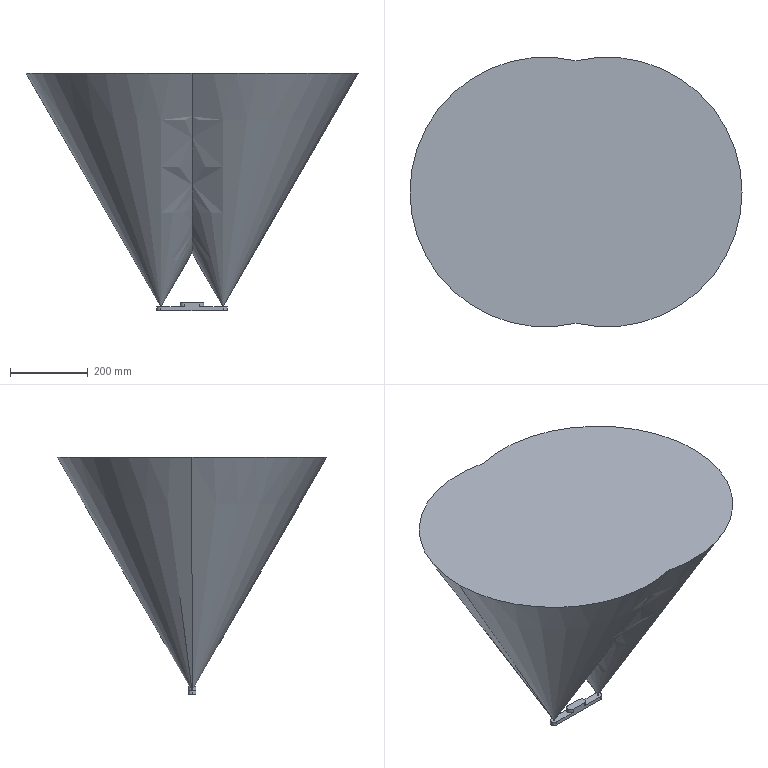Part | SolidWorks | features Revolution 2, Cut 1, Extrusion 1, Fillet 1, HoleWzd 1, ICE 1 | 2 solids | 40 faces | box 852.82 x 692.82 x 610 mm | volume 106933293 mm3 | cylinder 19 | cone 12 | plane 9 | commonest cylinder face diameters 1.6 x8 20 x7 2 x4
STEP:
#1=CARTESIAN_POINT('',(9.,10.,8.));
#2=VERTEX_POINT('',#1);
#3=CARTESIAN_POINT('',(11.,10.,8.));
#4=VERTEX_POINT('',#3);
#5=CARTESIAN_POINT('',(10.,10.,8.));
#6=DIRECTION('',(0.,0.,1.));
#7=DIRECTION('',(1.,0.,0.));
#8=AXIS2_PLACEMENT_3D('',#5,#6,#7);
#9=CIRCLE('',#8,1.);
#10=EDGE_CURVE('',#2,#4,#9,.T.);
#11=ORIENTED_EDGE('',*,*,#10,.F.);
#12=CARTESIAN_POINT('',(9.,10.,10.));
#13=VERTEX_POINT('',#12);
#14=CARTESIAN_POINT('',(9.,10.,8.));
#15=DIRECTION('',(0.,0.,1.));
#16=VECTOR('',#15,1000.);
#17=LINE('',#14,#16);
#18=EDGE_CURVE('',#2,#13,#17,.T.);
#19=ORIENTED_EDGE('',*,*,#18,.T.);
#20=CARTESIAN_POINT('',(11.,10.,10.));
#21=VERTEX_POINT('',#20);
#22=CARTESIAN_POINT('',(10.,10.,10.));
#23=DIRECTION('',(0.,0.,1.));
#24=DIRECTION('',(1.,0.,0.));
#25=AXIS2_PLACEMENT_3D('',#22,#23,#24);
#26=CIRCLE('',#25,1.);
#27=EDGE_CURVE('',#13,#21,#26,.T.);
#28=ORIENTED_EDGE('',*,*,#27,.T.);
#29=CARTESIAN_POINT('',(11.,10.,8.));
#30=DIRECTION('',(0.,0.,1.));
#31=VECTOR('',#30,1000.);
#32=LINE('',#29,#31);
#33=EDGE_CURVE('',#4,#21,#32,.T.);
#34=ORIENTED_EDGE('',*,*,#33,.F.);
#35=EDGE_LOOP('',(#11,#19,#28,#34));
#36=FACE_OUTER_BOUND('',#35,.T.);
#37=CARTESIAN_POINT('',(10.,10.,8.));
#38=DIRECTION('',(0.,0.,1.));
#39=DIRECTION('',(1.,0.,0.));
#40=AXIS2_PLACEMENT_3D('',#37,#38,#39);
#41=CYLINDRICAL_SURFACE('',#40,1.);
#42=ADVANCED_FACE('',(#36),#41,.F.);
#43=CARTESIAN_POINT('',(169.,10.,8.));
#44=VERTEX_POINT('',#43);
#45=CARTESIAN_POINT('',(171.,10.,8.));
#46=VERTEX_POINT('',#45);
#47=CARTESIAN_POINT('',(170.,10.,8.));
#48=DIRECTION('',(0.,0.,1.));
#49=DIRECTION('',(1.,0.,0.));
#50=AXIS2_PLACEMENT_3D('',#47,#48,#49);
#51=CIRCLE('',#50,1.);
#52=EDGE_CURVE('',#44,#46,#51,.T.);
#53=ORIENTED_EDGE('',*,*,#52,.F.);
#54=CARTESIAN_POINT('',(169.,10.,10.));
#55=VERTEX_POINT('',#54);
#56=CARTESIAN_POINT('',(169.,10.,8.));
#57=DIRECTION('',(0.,0.,1.));
#58=VECTOR('',#57,1000.);
#59=LINE('',#56,#58);
#60=EDGE_CURVE('',#44,#55,#59,.T.);
#61=ORIENTED_EDGE('',*,*,#60,.T.);
#62=CARTESIAN_POINT('',(171.,10.,10.));
#63=VERTEX_POINT('',#62);
#64=CARTESIAN_POINT('',(170.,10.,10.));
#65=DIRECTION('',(0.,0.,1.));
#66=DIRECTION('',(1.,0.,0.));
#67=AXIS2_PLACEMENT_3D('',#64,#65,#66);
#68=CIRCLE('',#67,1.);
#69=EDGE_CURVE('',#55,#63,#68,.T.);
#70=ORIENTED_EDGE('',*,*,#69,.T.);
#71=CARTESIAN_POINT('',(171.,10.,8.));
#72=DIRECTION('',(0.,0.,1.));
#73=VECTOR('',#72,1000.);
#74=LINE('',#71,#73);
#75=EDGE_CURVE('',#46,#63,#74,.T.);
#76=ORIENTED_EDGE('',*,*,#75,.F.);
#77=EDGE_LOOP('',(#53,#61,#70,#76));
#78=FACE_OUTER_BOUND('',#77,.T.);
#79=CARTESIAN_POINT('',(170.,10.,8.));
#80=DIRECTION('',(0.,0.,1.));
#81=DIRECTION('',(1.,0.,0.));
#82=AXIS2_PLACEMENT_3D('',#79,#80,#81);
#83=CYLINDRICAL_SURFACE('',#82,1.);
#84=ADVANCED_FACE('',(#78),#83,.F.);
#85=CARTESIAN_POINT('',(60.,10.,20.));
#86=VERTEX_POINT('',#85);
#87=CARTESIAN_POINT('',(70.,0.,20.));
#88=VERTEX_POINT('',#87);
#89=CARTESIAN_POINT('',(70.,10.,20.));
#90=DIRECTION('',(0.,0.,1.));
#91=DIRECTION('',(1.,0.,0.));
#92=AXIS2_PLACEMENT_3D('',#89,#90,#91);
#93=CIRCLE('',#92,10.);
#94=EDGE_CURVE('',#86,#88,#93,.T.);
#95=ORIENTED_EDGE('',*,*,#94,.F.);
#96=CARTESIAN_POINT('',(60.,10.,10.));
#97=VERTEX_POINT('',#96);
#98=CARTESIAN_POINT('',(60.,10.,20.));
#99=DIRECTION('',(0.,0.,-1.));
#100=VECTOR('',#99,1000.);
#101=LINE('',#98,#100);
#102=EDGE_CURVE('',#86,#97,#101,.T.);
#103=ORIENTED_EDGE('',*,*,#102,.T.);
#104=CARTESIAN_POINT('',(70.,0.,10.));
#105=VERTEX_POINT('',#104);
#106=CARTESIAN_POINT('',(70.,10.,10.));
#107=DIRECTION('',(0.,0.,1.));
#108=DIRECTION('',(1.,0.,0.));
#109=AXIS2_PLACEMENT_3D('',#106,#107,#108);
#110=CIRCLE('',#109,10.);
#111=EDGE_CURVE('',#97,#105,#110,.T.);
#112=ORIENTED_EDGE('',*,*,#111,.T.);
#113=CARTESIAN_POINT('',(70.,0.,20.));
#114=DIRECTION('',(0.,0.,-1.));
#115=VECTOR('',#114,1000.);
#116=LINE('',#113,#115);
#117=EDGE_CURVE('',#88,#105,#116,.T.);
#118=ORIENTED_EDGE('',*,*,#117,.F.);
#119=EDGE_LOOP('',(#95,#103,#112,#118));
#120=FACE_OUTER_BOUND('',#119,.T.);
#121=CARTESIAN_POINT('',(70.,10.,20.));
#122=DIRECTION('',(0.,0.,-1.));
#123=DIRECTION('',(-1.,0.,0.));
#124=AXIS2_PLACEMENT_3D('',#121,#122,#123);
#125=CYLINDRICAL_SURFACE('',#124,10.);
#126=ADVANCED_FACE('',(#120),#125,.T.);
#127=CARTESIAN_POINT('',(155.8,16.,5.2));
#128=VERTEX_POINT('',#127);
#129=CARTESIAN_POINT('',(154.2,16.,5.2));
#130=VERTEX_POINT('',#129);
#131=CARTESIAN_POINT('',(155.,16.,5.2));
#132=DIRECTION('',(0.,0.,-1.));
#133=DIRECTION('',(-1.,0.,0.));
#134=AXIS2_PLACEMENT_3D('',#131,#132,#133);
#135=CIRCLE('',#134,0.8);
#136=EDGE_CURVE('',#128,#130,#135,.T.);
#137=ORIENTED_EDGE('',*,*,#136,.F.);
#138=CARTESIAN_POINT('',(155.8,16.,0.));
#139=VERTEX_POINT('',#138);
#140=CARTESIAN_POINT('',(155.8,16.,0.));
#141=DIRECTION('',(0.,0.,-1.));
#142=VECTOR('',#141,1000.);
#143=LINE('',#140,#142);
#144=EDGE_CURVE('',#128,#139,#143,.T.);
#145=ORIENTED_EDGE('',*,*,#144,.T.);
#146=CARTESIAN_POINT('',(154.2,16.,0.));
#147=VERTEX_POINT('',#146);
#148=CARTESIAN_POINT('',(155.,16.,0.));
#149=DIRECTION('',(0.,0.,-1.));
#150=DIRECTION('',(-1.,0.,0.));
#151=AXIS2_PLACEMENT_3D('',#148,#149,#150);
#152=CIRCLE('',#151,0.8);
#153=EDGE_CURVE('',#139,#147,#152,.T.);
#154=ORIENTED_EDGE('',*,*,#153,.T.);
#155=CARTESIAN_POINT('',(154.2,16.,0.));
#156=DIRECTION('',(0.,0.,-1.));
#157=VECTOR('',#156,1000.);
#158=LINE('',#155,#157);
#159=EDGE_CURVE('',#130,#147,#158,.T.);
#160=ORIENTED_EDGE('',*,*,#159,.F.);
#161=EDGE_LOOP('',(#137,#145,#154,#160));
#162=FACE_OUTER_BOUND('',#161,.T.);
#163=CARTESIAN_POINT('',(155.,16.,0.));
#164=DIRECTION('',(0.,0.,-1.));
#165=DIRECTION('',(-1.,0.,0.));
#166=AXIS2_PLACEMENT_3D('',#163,#164,#165);
#167=CYLINDRICAL_SURFACE('',#166,0.8);
#168=ADVANCED_FACE('',(#162),#167,.F.);
#169=CARTESIAN_POINT('',(155.,16.,5.681));
#170=VERTEX_POINT('',#169);
#171=CARTESIAN_POINT('',(154.2,16.,5.2));
#172=DIRECTION('',(-0.8572,0.,-0.515));
#173=VECTOR('',#172,1000.);
#174=LINE('',#171,#173);
#175=EDGE_CURVE('',#170,#130,#174,.T.);
#176=ORIENTED_EDGE('',*,*,#175,.F.);
#177=CARTESIAN_POINT('',(155.8,16.,5.2));
#178=DIRECTION('',(0.8572,0.,-0.515));
#179=VECTOR('',#178,1000.);
#180=LINE('',#177,#179);
#181=EDGE_CURVE('',#170,#128,#180,.T.);
#182=ORIENTED_EDGE('',*,*,#181,.T.);
#183=ORIENTED_EDGE('',*,*,#136,.T.);
#184=EDGE_LOOP('',(#176,#182,#183));
#185=FACE_OUTER_BOUND('',#184,.T.);
#186=CARTESIAN_POINT('',(155.,16.,5.2));
#187=DIRECTION('',(0.,0.,-1.));
#188=DIRECTION('',(-1.,0.,0.));
#189=AXIS2_PLACEMENT_3D('',#186,#187,#188);
#190=CONICAL_SURFACE('',#189,0.8,1.03);
#191=ADVANCED_FACE('',(#185),#190,.F.);
#192=CARTESIAN_POINT('',(155.8,4.,5.2));
#193=VERTEX_POINT('',#192);
#194=CARTESIAN_POINT('',(154.2,4.,5.2));
#195=VERTEX_POINT('',#194);
#196=CARTESIAN_POINT('',(155.,4.,5.2));
#197=DIRECTION('',(0.,0.,-1.));
#198=DIRECTION('',(-1.,0.,0.));
#199=AXIS2_PLACEMENT_3D('',#196,#197,#198);
#200=CIRCLE('',#199,0.8);
#201=EDGE_CURVE('',#193,#195,#200,.T.);
#202=ORIENTED_EDGE('',*,*,#201,.F.);
#203=CARTESIAN_POINT('',(155.8,4.,0.));
#204=VERTEX_POINT('',#203);
#205=CARTESIAN_POINT('',(155.8,4.,0.));
#206=DIRECTION('',(0.,0.,-1.));
#207=VECTOR('',#206,1000.);
#208=LINE('',#205,#207);
#209=EDGE_CURVE('',#193,#204,#208,.T.);
#210=ORIENTED_EDGE('',*,*,#209,.T.);
#211=CARTESIAN_POINT('',(154.2,4.,0.));
#212=VERTEX_POINT('',#211);
#213=CARTESIAN_POINT('',(155.,4.,0.));
#214=DIRECTION('',(0.,0.,-1.));
#215=DIRECTION('',(-1.,0.,0.));
#216=AXIS2_PLACEMENT_3D('',#213,#214,#215);
#217=CIRCLE('',#216,0.8);
#218=EDGE_CURVE('',#204,#212,#217,.T.);
#219=ORIENTED_EDGE('',*,*,#218,.T.);
#220=CARTESIAN_POINT('',(154.2,4.,0.));
#221=DIRECTION('',(0.,0.,-1.));
#222=VECTOR('',#221,1000.);
#223=LINE('',#220,#222);
#224=EDGE_CURVE('',#195,#212,#223,.T.);
#225=ORIENTED_EDGE('',*,*,#224,.F.);
#226=EDGE_LOOP('',(#202,#210,#219,#225));
#227=FACE_OUTER_BOUND('',#226,.T.);
#228=CARTESIAN_POINT('',(155.,4.,0.));
#229=DIRECTION('',(0.,0.,-1.));
#230=DIRECTION('',(-1.,0.,0.));
#231=AXIS2_PLACEMENT_3D('',#228,#229,#230);
#232=CYLINDRICAL_SURFACE('',#231,0.8);
#233=ADVANCED_FACE('',(#227),#232,.F.);
#234=CARTESIAN_POINT('',(155.,4.,5.681));
#235=VERTEX_POINT('',#234);
#236=CARTESIAN_POINT('',(154.2,4.,5.2));
#237=DIRECTION('',(-0.8572,0.,-0.515));
#238=VECTOR('',#237,1000.);
#239=LINE('',#236,#238);
#240=EDGE_CURVE('',#235,#195,#239,.T.);
#241=ORIENTED_EDGE('',*,*,#240,.F.);
#242=CARTESIAN_POINT('',(155.8,4.,5.2));
#243=DIRECTION('',(0.8572,0.,-0.515));
#244=VECTOR('',#243,1000.);
#245=LINE('',#242,#244);
#246=EDGE_CURVE('',#235,#193,#245,.T.);
#247=ORIENTED_EDGE('',*,*,#246,.T.);
#248=ORIENTED_EDGE('',*,*,#201,.T.);
#249=EDGE_LOOP('',(#241,#247,#248));
#250=FACE_OUTER_BOUND('',#249,.T.);
#251=CARTESIAN_POINT('',(155.,4.,5.2));
#252=DIRECTION('',(0.,0.,-1.));
#253=DIRECTION('',(-1.,0.,0.));
#254=AXIS2_PLACEMENT_3D('',#251,#252,#253);
#255=CONICAL_SURFACE('',#254,0.8,1.03);
#256=ADVANCED_FACE('',(#250),#255,.F.);
#257=CARTESIAN_POINT('',(25.8,16.,5.2));
#258=VERTEX_POINT('',#257);
#259=CARTESIAN_POINT('',(24.2,16.,5.2));
#260=VERTEX_POINT('',#259);
#261=CARTESIAN_POINT('',(25.,16.,5.2));
#262=DIRECTION('',(0.,0.,-1.));
#263=DIRECTION('',(-1.,0.,0.));
#264=AXIS2_PLACEMENT_3D('',#261,#262,#263);
#265=CIRCLE('',#264,0.8);
#266=EDGE_CURVE('',#258,#260,#265,.T.);
#267=ORIENTED_EDGE('',*,*,#266,.F.);
#268=CARTESIAN_POINT('',(25.8,16.,0.));
#269=VERTEX_POINT('',#268);
#270=CARTESIAN_POINT('',(25.8,16.,0.));
#271=DIRECTION('',(0.,0.,-1.));
#272=VECTOR('',#271,1000.);
#273=LINE('',#270,#272);
#274=EDGE_CURVE('',#258,#269,#273,.T.);
#275=ORIENTED_EDGE('',*,*,#274,.T.);
#276=CARTESIAN_POINT('',(24.2,16.,0.));
#277=VERTEX_POINT('',#276);
#278=CARTESIAN_POINT('',(25.,16.,0.));
#279=DIRECTION('',(0.,0.,-1.));
#280=DIRECTION('',(-1.,0.,0.));
#281=AXIS2_PLACEMENT_3D('',#278,#279,#280);
#282=CIRCLE('',#281,0.8);
#283=EDGE_CURVE('',#269,#277,#282,.T.);
#284=ORIENTED_EDGE('',*,*,#283,.T.);
#285=CARTESIAN_POINT('',(24.2,16.,0.));
#286=DIRECTION('',(0.,0.,-1.));
#287=VECTOR('',#286,1000.);
#288=LINE('',#285,#287);
#289=EDGE_CURVE('',#260,#277,#288,.T.);
#290=ORIENTED_EDGE('',*,*,#289,.F.);
#291=EDGE_LOOP('',(#267,#275,#284,#290));
#292=FACE_OUTER_BOUND('',#291,.T.);
#293=CARTESIAN_POINT('',(25.,16.,0.));
#294=DIRECTION('',(0.,0.,-1.));
#295=DIRECTION('',(-1.,0.,0.));
#296=AXIS2_PLACEMENT_3D('',#293,#294,#295);
#297=CYLINDRICAL_SURFACE('',#296,0.8);
#298=ADVANCED_FACE('',(#292),#297,.F.);
#299=CARTESIAN_POINT('',(25.,16.,5.681));
#300=VERTEX_POINT('',#299);
#301=CARTESIAN_POINT('',(24.2,16.,5.2));
#302=DIRECTION('',(-0.8572,0.,-0.515));
#303=VECTOR('',#302,1000.);
#304=LINE('',#301,#303);
#305=EDGE_CURVE('',#300,#260,#304,.T.);
#306=ORIENTED_EDGE('',*,*,#305,.F.);
#307=CARTESIAN_POINT('',(25.8,16.,5.2));
#308=DIRECTION('',(0.8572,0.,-0.515));
#309=VECTOR('',#308,1000.);
#310=LINE('',#307,#309);
#311=EDGE_CURVE('',#300,#258,#310,.T.);
#312=ORIENTED_EDGE('',*,*,#311,.T.);
#313=ORIENTED_EDGE('',*,*,#266,.T.);
#314=EDGE_LOOP('',(#306,#312,#313));
#315=FACE_OUTER_BOUND('',#314,.T.);
#316=CARTESIAN_POINT('',(25.,16.,5.2));
#317=DIRECTION('',(0.,0.,-1.));
#318=DIRECTION('',(-1.,0.,0.));
#319=AXIS2_PLACEMENT_3D('',#316,#317,#318);
#320=CONICAL_SURFACE('',#319,0.8,1.03);
#321=ADVANCED_FACE('',(#315),#320,.F.);
#322=CARTESIAN_POINT('',(25.8,4.,5.2));
#323=VERTEX_POINT('',#322);
#324=CARTESIAN_POINT('',(24.2,4.,5.2));
#325=VERTEX_POINT('',#324);
#326=CARTESIAN_POINT('',(25.,4.,5.2));
#327=DIRECTION('',(0.,0.,-1.));
#328=DIRECTION('',(-1.,0.,0.));
#329=AXIS2_PLACEMENT_3D('',#326,#327,#328);
#330=CIRCLE('',#329,0.8);
#331=EDGE_CURVE('',#323,#325,#330,.T.);
#332=ORIENTED_EDGE('',*,*,#331,.F.);
#333=CARTESIAN_POINT('',(25.8,4.,0.));
#334=VERTEX_POINT('',#333);
#335=CARTESIAN_POINT('',(25.8,4.,0.));
#336=DIRECTION('',(0.,0.,-1.));
#337=VECTOR('',#336,1000.);
#338=LINE('',#335,#337);
#339=EDGE_CURVE('',#323,#334,#338,.T.);
#340=ORIENTED_EDGE('',*,*,#339,.T.);
#341=CARTESIAN_POINT('',(24.2,4.,0.));
#342=VERTEX_POINT('',#341);
#343=CARTESIAN_POINT('',(25.,4.,0.));
#344=DIRECTION('',(0.,0.,-1.));
#345=DIRECTION('',(-1.,0.,0.));
#346=AXIS2_PLACEMENT_3D('',#343,#344,#345);
#347=CIRCLE('',#346,0.8);
#348=EDGE_CURVE('',#334,#342,#347,.T.);
#349=ORIENTED_EDGE('',*,*,#348,.T.);
#350=CARTESIAN_POINT('',(24.2,4.,0.));
#351=DIRECTION('',(0.,0.,-1.));
#352=VECTOR('',#351,1000.);
#353=LINE('',#350,#352);
#354=EDGE_CURVE('',#325,#342,#353,.T.);
#355=ORIENTED_EDGE('',*,*,#354,.F.);
#356=EDGE_LOOP('',(#332,#340,#349,#355));
#357=FACE_OUTER_BOUND('',#356,.T.);
#358=CARTESIAN_POINT('',(25.,4.,0.));
#359=DIRECTION('',(0.,0.,-1.));
#360=DIRECTION('',(-1.,0.,0.));
#361=AXIS2_PLACEMENT_3D('',#358,#359,#360);
#362=CYLINDRICAL_SURFACE('',#361,0.8);
#363=ADVANCED_FACE('',(#357),#362,.F.);
#364=CARTESIAN_POINT('',(25.,4.,5.681));
#365=VERTEX_POINT('',#364);
#366=CARTESIAN_POINT('',(24.2,4.,5.2));
#367=DIRECTION('',(-0.8572,0.,-0.515));
#368=VECTOR('',#367,1000.);
#369=LINE('',#366,#368);
#370=EDGE_CURVE('',#365,#325,#369,.T.);
#371=ORIENTED_EDGE('',*,*,#370,.F.);
#372=CARTESIAN_POINT('',(25.8,4.,5.2));
#373=DIRECTION('',(0.8572,0.,-0.515));
#374=VECTOR('',#373,1000.);
#375=LINE('',#372,#374);
#376=EDGE_CURVE('',#365,#323,#375,.T.);
#377=ORIENTED_EDGE('',*,*,#376,.T.);
#378=ORIENTED_EDGE('',*,*,#331,.T.);
#379=EDGE_LOOP('',(#371,#377,#378));
#380=FACE_OUTER_BOUND('',#379,.T.);
#381=CARTESIAN_POINT('',(25.,4.,5.2));
#382=DIRECTION('',(0.,0.,-1.));
#383=DIRECTION('',(-1.,0.,0.));
#384=AXIS2_PLACEMENT_3D('',#381,#382,#383);
#385=CONICAL_SURFACE('',#384,0.8,1.03);
#386=ADVANCED_FACE('',(#380),#385,.F.);
#387=CARTESIAN_POINT('',(10.,10.,10.));
#388=DIRECTION('',(0.,0.,1.));
#389=DIRECTION('',(1.,0.,0.));
#390=AXIS2_PLACEMENT_3D('',#387,#388,#389);
#391=CIRCLE('',#390,1.);
#392=EDGE_CURVE('',#21,#13,#391,.T.);
#393=ORIENTED_EDGE('',*,*,#392,.F.);
#394=ORIENTED_EDGE('',*,*,#27,.F.);
#395=EDGE_LOOP('',(#393,#394));
#396=FACE_BOUND('',#395,.T.);
#397=CARTESIAN_POINT('',(70.,20.,10.));
#398=VERTEX_POINT('',#397);
#399=CARTESIAN_POINT('',(70.,10.,10.));
#400=DIRECTION('',(0.,0.,1.));
#401=DIRECTION('',(1.,0.,0.));
#402=AXIS2_PLACEMENT_3D('',#399,#400,#401);
#403=CIRCLE('',#402,10.);
#404=EDGE_CURVE('',#398,#97,#403,.T.);
#405=ORIENTED_EDGE('',*,*,#404,.F.);
#406=CARTESIAN_POINT('',(10.,20.,10.));
#407=VERTEX_POINT('',#406);
#408=CARTESIAN_POINT('',(0.,20.,10.));
#409=DIRECTION('',(-1.,0.,0.));
#410=VECTOR('',#409,1000.);
#411=LINE('',#408,#410);
#412=EDGE_CURVE('',#398,#407,#411,.T.);
#413=ORIENTED_EDGE('',*,*,#412,.T.);
#414=CARTESIAN_POINT('',(0.,10.,10.));
#415=VERTEX_POINT('',#414);
#416=CARTESIAN_POINT('',(10.,10.,10.));
#417=DIRECTION('',(0.,0.,1.));
#418=DIRECTION('',(-1.,0.,0.));
#419=AXIS2_PLACEMENT_3D('',#416,#417,#418);
#420=CIRCLE('',#419,10.);
#421=EDGE_CURVE('',#407,#415,#420,.T.);
#422=ORIENTED_EDGE('',*,*,#421,.T.);
#423=CARTESIAN_POINT('',(10.,0.,10.));
#424=VERTEX_POINT('',#423);
#425=CARTESIAN_POINT('',(10.,10.,10.));
#426=DIRECTION('',(0.,0.,1.));
#427=DIRECTION('',(-1.,0.,0.));
#428=AXIS2_PLACEMENT_3D('',#425,#426,#427);
#429=CIRCLE('',#428,10.);
#430=EDGE_CURVE('',#415,#424,#429,.T.);
#431=ORIENTED_EDGE('',*,*,#430,.T.);
#432=CARTESIAN_POINT('',(0.,0.,10.));
#433=DIRECTION('',(1.,0.,0.));
#434=VECTOR('',#433,1000.);
#435=LINE('',#432,#434);
#436=EDGE_CURVE('',#424,#105,#435,.T.);
#437=ORIENTED_EDGE('',*,*,#436,.T.);
#438=ORIENTED_EDGE('',*,*,#111,.F.);
#439=EDGE_LOOP('',(#405,#413,#422,#431,#437,#438));
#440=FACE_OUTER_BOUND('',#439,.T.);
#441=CARTESIAN_POINT('',(0.,0.,10.));
#442=DIRECTION('',(0.,0.,-1.));
#443=DIRECTION('',(-1.,0.,0.));
#444=AXIS2_PLACEMENT_3D('',#441,#442,#443);
#445=PLANE('',#444);
#446=ADVANCED_FACE('',(#396,#440),#445,.F.);
#447=CARTESIAN_POINT('',(10.,0.,0.));
#448=VERTEX_POINT('',#447);
#449=CARTESIAN_POINT('',(170.,0.,0.));
#450=VERTEX_POINT('',#449);
#451=CARTESIAN_POINT('',(0.,0.,0.));
#452=DIRECTION('',(1.,0.,0.));
#453=VECTOR('',#452,1000.);
#454=LINE('',#451,#453);
#455=EDGE_CURVE('',#448,#450,#454,.T.);
#456=ORIENTED_EDGE('',*,*,#455,.T.);
#457=CARTESIAN_POINT('',(170.,0.,10.));
#458=VERTEX_POINT('',#457);
#459=CARTESIAN_POINT('',(170.,0.,10.));
#460=DIRECTION('',(0.,0.,1.));
#461=VECTOR('',#460,1000.);
#462=LINE('',#459,#461);
#463=EDGE_CURVE('',#450,#458,#462,.T.);
#464=ORIENTED_EDGE('',*,*,#463,.T.);
#465=CARTESIAN_POINT('',(110.,0.,10.));
#466=VERTEX_POINT('',#465);
#467=CARTESIAN_POINT('',(0.,0.,10.));
#468=DIRECTION('',(1.,0.,0.));
#469=VECTOR('',#468,1000.);
#470=LINE('',#467,#469);
#471=EDGE_CURVE('',#466,#458,#470,.T.);
#472=ORIENTED_EDGE('',*,*,#471,.F.);
#473=CARTESIAN_POINT('',(110.,0.,20.));
#474=VERTEX_POINT('',#473);
#475=CARTESIAN_POINT('',(110.,0.,20.));
#476=DIRECTION('',(0.,0.,-1.));
#477=VECTOR('',#476,1000.);
#478=LINE('',#475,#477);
#479=EDGE_CURVE('',#474,#466,#478,.T.);
#480=ORIENTED_EDGE('',*,*,#479,.F.);
#481=CARTESIAN_POINT('',(70.,0.,20.));
#482=DIRECTION('',(1.,0.,0.));
#483=VECTOR('',#482,1000.);
#484=LINE('',#481,#483);
#485=EDGE_CURVE('',#88,#474,#484,.T.);
#486=ORIENTED_EDGE('',*,*,#485,.F.);
#487=ORIENTED_EDGE('',*,*,#117,.T.);
#488=ORIENTED_EDGE('',*,*,#436,.F.);
#489=CARTESIAN_POINT('',(10.,0.,10.));
#490=DIRECTION('',(0.,0.,-1.));
#491=VECTOR('',#490,1000.);
#492=LINE('',#489,#491);
#493=EDGE_CURVE('',#424,#448,#492,.T.);
#494=ORIENTED_EDGE('',*,*,#493,.T.);
#495=EDGE_LOOP('',(#456,#464,#472,#480,#486,#487,#488,#494));
#496=FACE_OUTER_BOUND('',#495,.T.);
#497=CARTESIAN_POINT('',(0.,0.,10.));
#498=DIRECTION('',(0.,1.,0.));
#499=DIRECTION('',(0.,0.,1.));
#500=AXIS2_PLACEMENT_3D('',#497,#498,#499);
#501=PLANE('',#500);
#502=ADVANCED_FACE('',(#496),#501,.F.);
#503=CARTESIAN_POINT('',(170.,20.,10.));
#504=VERTEX_POINT('',#503);
#505=CARTESIAN_POINT('',(110.,20.,10.));
#506=VERTEX_POINT('',#505);
#507=CARTESIAN_POINT('',(0.,20.,10.));
#508=DIRECTION('',(-1.,0.,0.));
#509=VECTOR('',#508,1000.);
#510=LINE('',#507,#509);
#511=EDGE_CURVE('',#504,#506,#510,.T.);
#512=ORIENTED_EDGE('',*,*,#511,.F.);
#513=CARTESIAN_POINT('',(170.,20.,0.));
#514=VERTEX_POINT('',#513);
#515=CARTESIAN_POINT('',(170.,20.,10.));
#516=DIRECTION('',(0.,0.,-1.));
#517=VECTOR('',#516,1000.);
#518=LINE('',#515,#517);
#519=EDGE_CURVE('',#504,#514,#518,.T.);
#520=ORIENTED_EDGE('',*,*,#519,.T.);
#521=CARTESIAN_POINT('',(10.,20.,0.));
#522=VERTEX_POINT('',#521);
#523=CARTESIAN_POINT('',(0.,20.,0.));
#524=DIRECTION('',(-1.,0.,0.));
#525=VECTOR('',#524,1000.);
#526=LINE('',#523,#525);
#527=EDGE_CURVE('',#514,#522,#526,.T.);
#528=ORIENTED_EDGE('',*,*,#527,.T.);
#529=CARTESIAN_POINT('',(10.,20.,10.));
#530=DIRECTION('',(0.,0.,1.));
#531=VECTOR('',#530,1000.);
#532=LINE('',#529,#531);
#533=EDGE_CURVE('',#522,#407,#532,.T.);
#534=ORIENTED_EDGE('',*,*,#533,.T.);
#535=ORIENTED_EDGE('',*,*,#412,.F.);
#536=CARTESIAN_POINT('',(70.,20.,20.));
#537=VERTEX_POINT('',#536);
#538=CARTESIAN_POINT('',(70.,20.,20.));
#539=DIRECTION('',(0.,0.,-1.));
#540=VECTOR('',#539,1000.);
#541=LINE('',#538,#540);
#542=EDGE_CURVE('',#537,#398,#541,.T.);
#543=ORIENTED_EDGE('',*,*,#542,.F.);
#544=CARTESIAN_POINT('',(110.,20.,20.));
#545=VERTEX_POINT('',#544);
#546=CARTESIAN_POINT('',(70.,20.,20.));
#547=DIRECTION('',(-1.,0.,0.));
#548=VECTOR('',#547,1000.);
#549=LINE('',#546,#548);
#550=EDGE_CURVE('',#545,#537,#549,.T.);
#551=ORIENTED_EDGE('',*,*,#550,.F.);
#552=CARTESIAN_POINT('',(110.,20.,20.));
#553=DIRECTION('',(0.,0.,-1.));
#554=VECTOR('',#553,1000.);
#555=LINE('',#552,#554);
#556=EDGE_CURVE('',#545,#506,#555,.T.);
#557=ORIENTED_EDGE('',*,*,#556,.T.);
#558=EDGE_LOOP('',(#512,#520,#528,#534,#535,#543,#551,#557));
#559=FACE_OUTER_BOUND('',#558,.T.);
#560=CARTESIAN_POINT('',(0.,20.,10.));
#561=DIRECTION('',(0.,-1.,0.));
#562=DIRECTION('',(0.,0.,-1.));
#563=AXIS2_PLACEMENT_3D('',#560,#561,#562);
#564=PLANE('',#563);
#565=ADVANCED_FACE('',(#559),#564,.F.);
#566=CARTESIAN_POINT('',(170.,10.,10.));
#567=DIRECTION('',(0.,0.,1.));
#568=DIRECTION('',(1.,0.,0.));
#569=AXIS2_PLACEMENT_3D('',#566,#567,#568);
#570=CIRCLE('',#569,1.);
#571=EDGE_CURVE('',#63,#55,#570,.T.);
#572=ORIENTED_EDGE('',*,*,#571,.F.);
#573=ORIENTED_EDGE('',*,*,#69,.F.);
#574=EDGE_LOOP('',(#572,#573));
#575=FACE_BOUND('',#574,.T.);
#576=CARTESIAN_POINT('',(110.,10.,10.));
#577=DIRECTION('',(0.,0.,1.));
#578=DIRECTION('',(1.,0.,0.));
#579=AXIS2_PLACEMENT_3D('',#576,#577,#578);
#580=CIRCLE('',#579,10.);
#581=EDGE_CURVE('',#466,#506,#580,.T.);
#582=ORIENTED_EDGE('',*,*,#581,.F.);
#583=ORIENTED_EDGE('',*,*,#471,.T.);
#584=CARTESIAN_POINT('',(180.,10.,10.));
#585=VERTEX_POINT('',#584);
#586=CARTESIAN_POINT('',(170.,10.,10.));
#587=DIRECTION('',(0.,0.,1.));
#588=DIRECTION('',(-1.,0.,0.));
#589=AXIS2_PLACEMENT_3D('',#586,#587,#588);
#590=CIRCLE('',#589,10.);
#591=EDGE_CURVE('',#458,#585,#590,.T.);
#592=ORIENTED_EDGE('',*,*,#591,.T.);
#593=CARTESIAN_POINT('',(170.,10.,10.));
#594=DIRECTION('',(0.,0.,1.));
#595=DIRECTION('',(-1.,0.,0.));
#596=AXIS2_PLACEMENT_3D('',#593,#594,#595);
#597=CIRCLE('',#596,10.);
#598=EDGE_CURVE('',#585,#504,#597,.T.);
#599=ORIENTED_EDGE('',*,*,#598,.T.);
#600=ORIENTED_EDGE('',*,*,#511,.T.);
#601=EDGE_LOOP('',(#582,#583,#592,#599,#600));
#602=FACE_OUTER_BOUND('',#601,.T.);
#603=CARTESIAN_POINT('',(0.,0.,10.));
#604=DIRECTION('',(0.,0.,-1.));
#605=DIRECTION('',(-1.,0.,0.));
#606=AXIS2_PLACEMENT_3D('',#603,#604,#605);
#607=PLANE('',#606);
#608=ADVANCED_FACE('',(#575,#602),#607,.F.);
#609=CARTESIAN_POINT('',(155.,16.,0.));
#610=DIRECTION('',(0.,0.,-1.));
#611=DIRECTION('',(-1.,0.,0.));
#612=AXIS2_PLACEMENT_3D('',#609,#610,#611);
#613=CIRCLE('',#612,0.8);
#614=EDGE_CURVE('',#147,#139,#613,.T.);
#615=ORIENTED_EDGE('',*,*,#614,.F.);
#616=ORIENTED_EDGE('',*,*,#153,.F.);
#617=EDGE_LOOP('',(#615,#616));
#618=FACE_BOUND('',#617,.T.);
#619=CARTESIAN_POINT('',(155.,4.,0.));
#620=DIRECTION('',(0.,0.,-1.));
#621=DIRECTION('',(-1.,0.,0.));
#622=AXIS2_PLACEMENT_3D('',#619,#620,#621);
#623=CIRCLE('',#622,0.8);
#624=EDGE_CURVE('',#212,#204,#623,.T.);
#625=ORIENTED_EDGE('',*,*,#624,.F.);
#626=ORIENTED_EDGE('',*,*,#218,.F.);
#627=EDGE_LOOP('',(#625,#626));
#628=FACE_BOUND('',#627,.T.);
#629=CARTESIAN_POINT('',(25.,16.,0.));
#630=DIRECTION('',(0.,0.,-1.));
#631=DIRECTION('',(-1.,0.,0.));
#632=AXIS2_PLACEMENT_3D('',#629,#630,#631);
#633=CIRCLE('',#632,0.8);
#634=EDGE_CURVE('',#277,#269,#633,.T.);
#635=ORIENTED_EDGE('',*,*,#634,.F.);
#636=ORIENTED_EDGE('',*,*,#283,.F.);
#637=EDGE_LOOP('',(#635,#636));
#638=FACE_BOUND('',#637,.T.);
#639=CARTESIAN_POINT('',(25.,4.,0.));
#640=DIRECTION('',(0.,0.,-1.));
#641=DIRECTION('',(-1.,0.,0.));
#642=AXIS2_PLACEMENT_3D('',#639,#640,#641);
#643=CIRCLE('',#642,0.8);
#644=EDGE_CURVE('',#342,#334,#643,.T.);
#645=ORIENTED_EDGE('',*,*,#644,.F.);
#646=ORIENTED_EDGE('',*,*,#348,.F.);
#647=EDGE_LOOP('',(#645,#646));
#648=FACE_BOUND('',#647,.T.);
#649=CARTESIAN_POINT('',(180.,10.,0.));
#650=VERTEX_POINT('',#649);
#651=CARTESIAN_POINT('',(170.,10.,0.));
#652=DIRECTION('',(0.,0.,-1.));
#653=DIRECTION('',(-1.,0.,0.));
#654=AXIS2_PLACEMENT_3D('',#651,#652,#653);
#655=CIRCLE('',#654,10.);
#656=EDGE_CURVE('',#514,#650,#655,.T.);
#657=ORIENTED_EDGE('',*,*,#656,.T.);
#658=CARTESIAN_POINT('',(170.,10.,0.));
#659=DIRECTION('',(0.,0.,-1.));
#660=DIRECTION('',(-1.,0.,0.));
#661=AXIS2_PLACEMENT_3D('',#658,#659,#660);
#662=CIRCLE('',#661,10.);
#663=EDGE_CURVE('',#650,#450,#662,.T.);
#664=ORIENTED_EDGE('',*,*,#663,.T.);
#665=ORIENTED_EDGE('',*,*,#455,.F.);
#666=CARTESIAN_POINT('',(0.,10.,0.));
#667=VERTEX_POINT('',#666);
#668=CARTESIAN_POINT('',(10.,10.,0.));
#669=DIRECTION('',(0.,0.,-1.));
#670=DIRECTION('',(-1.,0.,0.));
#671=AXIS2_PLACEMENT_3D('',#668,#669,#670);
#672=CIRCLE('',#671,10.);
#673=EDGE_CURVE('',#448,#667,#672,.T.);
#674=ORIENTED_EDGE('',*,*,#673,.T.);
#675=CARTESIAN_POINT('',(10.,10.,0.));
#676=DIRECTION('',(0.,0.,-1.));
#677=DIRECTION('',(-1.,0.,0.));
#678=AXIS2_PLACEMENT_3D('',#675,#676,#677);
#679=CIRCLE('',#678,10.);
#680=EDGE_CURVE('',#667,#522,#679,.T.);
#681=ORIENTED_EDGE('',*,*,#680,.T.);
#682=ORIENTED_EDGE('',*,*,#527,.F.);
#683=EDGE_LOOP('',(#657,#664,#665,#674,#681,#682));
#684=FACE_OUTER_BOUND('',#683,.T.);
#685=CARTESIAN_POINT('',(0.,0.,0.));
#686=DIRECTION('',(0.,0.,-1.));
#687=DIRECTION('',(-1.,0.,0.));
#688=AXIS2_PLACEMENT_3D('',#685,#686,#687);
#689=PLANE('',#688);
#690=ADVANCED_FACE('',(#618,#628,#638,#648,#684),#689,.T.);
#691=ORIENTED_EDGE('',*,*,#519,.F.);
#692=ORIENTED_EDGE('',*,*,#598,.F.);
#693=CARTESIAN_POINT('',(180.,10.,10.));
#694=DIRECTION('',(0.,0.,1.));
#695=VECTOR('',#694,1000.);
#696=LINE('',#693,#695);
#697=EDGE_CURVE('',#650,#585,#696,.T.);
#698=ORIENTED_EDGE('',*,*,#697,.F.);
#699=ORIENTED_EDGE('',*,*,#656,.F.);
#700=EDGE_LOOP('',(#691,#692,#698,#699));
#701=FACE_OUTER_BOUND('',#700,.T.);
#702=CARTESIAN_POINT('',(170.,10.,10.));
#703=DIRECTION('',(0.,0.,-1.));
#704=DIRECTION('',(-1.,0.,0.));
#705=AXIS2_PLACEMENT_3D('',#702,#703,#704);
#706=CYLINDRICAL_SURFACE('',#705,10.);
#707=ADVANCED_FACE('',(#701),#706,.T.);
#708=ORIENTED_EDGE('',*,*,#591,.F.);
#709=ORIENTED_EDGE('',*,*,#463,.F.);
#710=ORIENTED_EDGE('',*,*,#663,.F.);
#711=ORIENTED_EDGE('',*,*,#697,.T.);
#712=EDGE_LOOP('',(#708,#709,#710,#711));
#713=FACE_OUTER_BOUND('',#712,.T.);
#714=CARTESIAN_POINT('',(170.,10.,10.));
#715=DIRECTION('',(0.,0.,-1.));
#716=DIRECTION('',(-1.,0.,0.));
#717=AXIS2_PLACEMENT_3D('',#714,#715,#716);
#718=CYLINDRICAL_SURFACE('',#717,10.);
#719=ADVANCED_FACE('',(#713),#718,.T.);
#720=CARTESIAN_POINT('',(0.,10.,10.));
#721=DIRECTION('',(0.,0.,-1.));
#722=VECTOR('',#721,1000.);
#723=LINE('',#720,#722);
#724=EDGE_CURVE('',#415,#667,#723,.T.);
#725=ORIENTED_EDGE('',*,*,#724,.F.);
#726=ORIENTED_EDGE('',*,*,#421,.F.);
#727=ORIENTED_EDGE('',*,*,#533,.F.);
#728=ORIENTED_EDGE('',*,*,#680,.F.);
#729=EDGE_LOOP('',(#725,#726,#727,#728));
#730=FACE_OUTER_BOUND('',#729,.T.);
#731=CARTESIAN_POINT('',(10.,10.,10.));
#732=DIRECTION('',(0.,0.,-1.));
#733=DIRECTION('',(-1.,0.,0.));
#734=AXIS2_PLACEMENT_3D('',#731,#732,#733);
#735=CYLINDRICAL_SURFACE('',#734,10.);
#736=ADVANCED_FACE('',(#730),#735,.T.);
#737=ORIENTED_EDGE('',*,*,#430,.F.);
#738=ORIENTED_EDGE('',*,*,#724,.T.);
#739=ORIENTED_EDGE('',*,*,#673,.F.);
#740=ORIENTED_EDGE('',*,*,#493,.F.);
#741=EDGE_LOOP('',(#737,#738,#739,#740));
#742=FACE_OUTER_BOUND('',#741,.T.);
#743=CARTESIAN_POINT('',(10.,10.,10.));
#744=DIRECTION('',(0.,0.,-1.));
#745=DIRECTION('',(-1.,0.,0.));
#746=AXIS2_PLACEMENT_3D('',#743,#744,#745);
#747=CYLINDRICAL_SURFACE('',#746,10.);
#748=ADVANCED_FACE('',(#742),#747,.T.);
#749=ORIENTED_EDGE('',*,*,#376,.F.);
#750=ORIENTED_EDGE('',*,*,#370,.T.);
#751=CARTESIAN_POINT('',(25.,4.,5.2));
#752=DIRECTION('',(0.,0.,-1.));
#753=DIRECTION('',(-1.,0.,0.));
#754=AXIS2_PLACEMENT_3D('',#751,#752,#753);
#755=CIRCLE('',#754,0.8);
#756=EDGE_CURVE('',#325,#323,#755,.T.);
#757=ORIENTED_EDGE('',*,*,#756,.T.);
#758=EDGE_LOOP('',(#749,#750,#757));
#759=FACE_OUTER_BOUND('',#758,.T.);
#760=CARTESIAN_POINT('',(25.,4.,5.2));
#761=DIRECTION('',(0.,0.,-1.));
#762=DIRECTION('',(-1.,0.,0.));
#763=AXIS2_PLACEMENT_3D('',#760,#761,#762);
#764=CONICAL_SURFACE('',#763,0.8,1.03);
#765=ADVANCED_FACE('',(#759),#764,.F.);
#766=ORIENTED_EDGE('',*,*,#339,.F.);
#767=ORIENTED_EDGE('',*,*,#756,.F.);
#768=ORIENTED_EDGE('',*,*,#354,.T.);
#769=ORIENTED_EDGE('',*,*,#644,.T.);
#770=EDGE_LOOP('',(#766,#767,#768,#769));
#771=FACE_OUTER_BOUND('',#770,.T.);
#772=CARTESIAN_POINT('',(25.,4.,0.));
#773=DIRECTION('',(0.,0.,-1.));
#774=DIRECTION('',(-1.,0.,0.));
#775=AXIS2_PLACEMENT_3D('',#772,#773,#774);
#776=CYLINDRICAL_SURFACE('',#775,0.8);
#777=ADVANCED_FACE('',(#771),#776,.F.);
#778=ORIENTED_EDGE('',*,*,#311,.F.);
#779=ORIENTED_EDGE('',*,*,#305,.T.);
#780=CARTESIAN_POINT('',(25.,16.,5.2));
#781=DIRECTION('',(0.,0.,-1.));
#782=DIRECTION('',(-1.,0.,0.));
#783=AXIS2_PLACEMENT_3D('',#780,#781,#782);
#784=CIRCLE('',#783,0.8);
#785=EDGE_CURVE('',#260,#258,#784,.T.);
#786=ORIENTED_EDGE('',*,*,#785,.T.);
#787=EDGE_LOOP('',(#778,#779,#786));
#788=FACE_OUTER_BOUND('',#787,.T.);
#789=CARTESIAN_POINT('',(25.,16.,5.2));
#790=DIRECTION('',(0.,0.,-1.));
#791=DIRECTION('',(-1.,0.,0.));
#792=AXIS2_PLACEMENT_3D('',#789,#790,#791);
#793=CONICAL_SURFACE('',#792,0.8,1.03);
#794=ADVANCED_FACE('',(#788),#793,.F.);
#795=ORIENTED_EDGE('',*,*,#274,.F.);
#796=ORIENTED_EDGE('',*,*,#785,.F.);
#797=ORIENTED_EDGE('',*,*,#289,.T.);
#798=ORIENTED_EDGE('',*,*,#634,.T.);
#799=EDGE_LOOP('',(#795,#796,#797,#798));
#800=FACE_OUTER_BOUND('',#799,.T.);
#801=CARTESIAN_POINT('',(25.,16.,0.));
#802=DIRECTION('',(0.,0.,-1.));
#803=DIRECTION('',(-1.,0.,0.));
#804=AXIS2_PLACEMENT_3D('',#801,#802,#803);
#805=CYLINDRICAL_SURFACE('',#804,0.8);
#806=ADVANCED_FACE('',(#800),#805,.F.);
#807=ORIENTED_EDGE('',*,*,#246,.F.);
#808=ORIENTED_EDGE('',*,*,#240,.T.);
#809=CARTESIAN_POINT('',(155.,4.,5.2));
#810=DIRECTION('',(0.,0.,-1.));
#811=DIRECTION('',(-1.,0.,0.));
#812=AXIS2_PLACEMENT_3D('',#809,#810,#811);
#813=CIRCLE('',#812,0.8);
#814=EDGE_CURVE('',#195,#193,#813,.T.);
#815=ORIENTED_EDGE('',*,*,#814,.T.);
#816=EDGE_LOOP('',(#807,#808,#815));
#817=FACE_OUTER_BOUND('',#816,.T.);
#818=CARTESIAN_POINT('',(155.,4.,5.2));
#819=DIRECTION('',(0.,0.,-1.));
#820=DIRECTION('',(-1.,0.,0.));
#821=AXIS2_PLACEMENT_3D('',#818,#819,#820);
#822=CONICAL_SURFACE('',#821,0.8,1.03);
#823=ADVANCED_FACE('',(#817),#822,.F.);
#824=ORIENTED_EDGE('',*,*,#209,.F.);
#825=ORIENTED_EDGE('',*,*,#814,.F.);
#826=ORIENTED_EDGE('',*,*,#224,.T.);
#827=ORIENTED_EDGE('',*,*,#624,.T.);
#828=EDGE_LOOP('',(#824,#825,#826,#827));
#829=FACE_OUTER_BOUND('',#828,.T.);
#830=CARTESIAN_POINT('',(155.,4.,0.));
#831=DIRECTION('',(0.,0.,-1.));
#832=DIRECTION('',(-1.,0.,0.));
#833=AXIS2_PLACEMENT_3D('',#830,#831,#832);
#834=CYLINDRICAL_SURFACE('',#833,0.8);
#835=ADVANCED_FACE('',(#829),#834,.F.);
#836=ORIENTED_EDGE('',*,*,#181,.F.);
#837=ORIENTED_EDGE('',*,*,#175,.T.);
#838=CARTESIAN_POINT('',(155.,16.,5.2));
#839=DIRECTION('',(0.,0.,-1.));
#840=DIRECTION('',(-1.,0.,0.));
#841=AXIS2_PLACEMENT_3D('',#838,#839,#840);
#842=CIRCLE('',#841,0.8);
#843=EDGE_CURVE('',#130,#128,#842,.T.);
#844=ORIENTED_EDGE('',*,*,#843,.T.);
#845=EDGE_LOOP('',(#836,#837,#844));
#846=FACE_OUTER_BOUND('',#845,.T.);
#847=CARTESIAN_POINT('',(155.,16.,5.2));
#848=DIRECTION('',(0.,0.,-1.));
#849=DIRECTION('',(-1.,0.,0.));
#850=AXIS2_PLACEMENT_3D('',#847,#848,#849);
#851=CONICAL_SURFACE('',#850,0.8,1.03);
#852=ADVANCED_FACE('',(#846),#851,.F.);
#853=ORIENTED_EDGE('',*,*,#144,.F.);
#854=ORIENTED_EDGE('',*,*,#843,.F.);
#855=ORIENTED_EDGE('',*,*,#159,.T.);
#856=ORIENTED_EDGE('',*,*,#614,.T.);
#857=EDGE_LOOP('',(#853,#854,#855,#856));
#858=FACE_OUTER_BOUND('',#857,.T.);
#859=CARTESIAN_POINT('',(155.,16.,0.));
#860=DIRECTION('',(0.,0.,-1.));
#861=DIRECTION('',(-1.,0.,0.));
#862=AXIS2_PLACEMENT_3D('',#859,#860,#861);
#863=CYLINDRICAL_SURFACE('',#862,0.8);
#864=ADVANCED_FACE('',(#858),#863,.F.);
#865=ORIENTED_EDGE('',*,*,#102,.F.);
#866=CARTESIAN_POINT('',(70.,10.,20.));
#867=DIRECTION('',(0.,0.,1.));
#868=DIRECTION('',(1.,0.,0.));
#869=AXIS2_PLACEMENT_3D('',#866,#867,#868);
#870=CIRCLE('',#869,10.);
#871=EDGE_CURVE('',#537,#86,#870,.T.);
#872=ORIENTED_EDGE('',*,*,#871,.F.);
#873=ORIENTED_EDGE('',*,*,#542,.T.);
#874=ORIENTED_EDGE('',*,*,#404,.T.);
#875=EDGE_LOOP('',(#865,#872,#873,#874));
#876=FACE_OUTER_BOUND('',#875,.T.);
#877=CARTESIAN_POINT('',(70.,10.,20.));
#878=DIRECTION('',(0.,0.,-1.));
#879=DIRECTION('',(-1.,0.,0.));
#880=AXIS2_PLACEMENT_3D('',#877,#878,#879);
#881=CYLINDRICAL_SURFACE('',#880,10.);
#882=ADVANCED_FACE('',(#876),#881,.T.);
#883=ORIENTED_EDGE('',*,*,#581,.T.);
#884=ORIENTED_EDGE('',*,*,#556,.F.);
#885=CARTESIAN_POINT('',(110.,10.,20.));
#886=DIRECTION('',(0.,0.,1.));
#887=DIRECTION('',(1.,0.,0.));
#888=AXIS2_PLACEMENT_3D('',#885,#886,#887);
#889=CIRCLE('',#888,10.);
#890=EDGE_CURVE('',#474,#545,#889,.T.);
#891=ORIENTED_EDGE('',*,*,#890,.F.);
#892=ORIENTED_EDGE('',*,*,#479,.T.);
#893=EDGE_LOOP('',(#883,#884,#891,#892));
#894=FACE_OUTER_BOUND('',#893,.T.);
#895=CARTESIAN_POINT('',(110.,10.,20.));
#896=DIRECTION('',(0.,0.,-1.));
#897=DIRECTION('',(-1.,0.,0.));
#898=AXIS2_PLACEMENT_3D('',#895,#896,#897);
#899=CYLINDRICAL_SURFACE('',#898,10.);
#900=ADVANCED_FACE('',(#894),#899,.T.);
#901=ORIENTED_EDGE('',*,*,#871,.T.);
#902=ORIENTED_EDGE('',*,*,#94,.T.);
#903=ORIENTED_EDGE('',*,*,#485,.T.);
#904=ORIENTED_EDGE('',*,*,#890,.T.);
#905=ORIENTED_EDGE('',*,*,#550,.T.);
#906=EDGE_LOOP('',(#901,#902,#903,#904,#905));
#907=FACE_OUTER_BOUND('',#906,.T.);
#908=CARTESIAN_POINT('',(70.,10.,20.));
#909=DIRECTION('',(0.,0.,1.));
#910=DIRECTION('',(1.,0.,0.));
#911=AXIS2_PLACEMENT_3D('',#908,#909,#910);
#912=PLANE('',#911);
#913=ADVANCED_FACE('',(#907),#912,.T.);
#914=ORIENTED_EDGE('',*,*,#60,.F.);
#915=CARTESIAN_POINT('',(170.,10.,8.));
#916=DIRECTION('',(0.,0.,1.));
#917=DIRECTION('',(1.,0.,0.));
#918=AXIS2_PLACEMENT_3D('',#915,#916,#917);
#919=CIRCLE('',#918,1.);
#920=EDGE_CURVE('',#46,#44,#919,.T.);
#921=ORIENTED_EDGE('',*,*,#920,.F.);
#922=ORIENTED_EDGE('',*,*,#75,.T.);
#923=ORIENTED_EDGE('',*,*,#571,.T.);
#924=EDGE_LOOP('',(#914,#921,#922,#923));
#925=FACE_OUTER_BOUND('',#924,.T.);
#926=CARTESIAN_POINT('',(170.,10.,8.));
#927=DIRECTION('',(0.,0.,1.));
#928=DIRECTION('',(1.,0.,0.));
#929=AXIS2_PLACEMENT_3D('',#926,#927,#928);
#930=CYLINDRICAL_SURFACE('',#929,1.);
#931=ADVANCED_FACE('',(#925),#930,.F.);
#932=ORIENTED_EDGE('',*,*,#920,.T.);
#933=ORIENTED_EDGE('',*,*,#52,.T.);
#934=EDGE_LOOP('',(#932,#933));
#935=FACE_OUTER_BOUND('',#934,.T.);
#936=CARTESIAN_POINT('',(170.,10.,8.));
#937=DIRECTION('',(0.,0.,1.));
#938=DIRECTION('',(1.,0.,0.));
#939=AXIS2_PLACEMENT_3D('',#936,#937,#938);
#940=PLANE('',#939);
#941=ADVANCED_FACE('',(#935),#940,.T.);
#942=ORIENTED_EDGE('',*,*,#18,.F.);
#943=CARTESIAN_POINT('',(10.,10.,8.));
#944=DIRECTION('',(0.,0.,1.));
#945=DIRECTION('',(1.,0.,0.));
#946=AXIS2_PLACEMENT_3D('',#943,#944,#945);
#947=CIRCLE('',#946,1.);
#948=EDGE_CURVE('',#4,#2,#947,.T.);
#949=ORIENTED_EDGE('',*,*,#948,.F.);
#950=ORIENTED_EDGE('',*,*,#33,.T.);
#951=ORIENTED_EDGE('',*,*,#392,.T.);
#952=EDGE_LOOP('',(#942,#949,#950,#951));
#953=FACE_OUTER_BOUND('',#952,.T.);
#954=CARTESIAN_POINT('',(10.,10.,8.));
#955=DIRECTION('',(0.,0.,1.));
#956=DIRECTION('',(1.,0.,0.));
#957=AXIS2_PLACEMENT_3D('',#954,#955,#956);
#958=CYLINDRICAL_SURFACE('',#957,1.);
#959=ADVANCED_FACE('',(#953),#958,.F.);
#960=ORIENTED_EDGE('',*,*,#948,.T.);
#961=ORIENTED_EDGE('',*,*,#10,.T.);
#962=EDGE_LOOP('',(#960,#961));
#963=FACE_OUTER_BOUND('',#962,.T.);
#964=CARTESIAN_POINT('',(10.,10.,8.));
#965=DIRECTION('',(0.,0.,1.));
#966=DIRECTION('',(1.,0.,0.));
#967=AXIS2_PLACEMENT_3D('',#964,#965,#966);
#968=PLANE('',#967);
#969=ADVANCED_FACE('',(#963),#968,.T.);
#970=CLOSED_SHELL('',(#42,#84,#126,#168,#191,#233,#256,#298,#321,#363,#386,#446,#502,#565,#608,#690,#707,#719,#736,#748,#765,#777,#794,#806,#823,#835,#852,#864,#882,#900,#913,#931,#941,#959,#969));
#971=MANIFOLD_SOLID_BREP('',#970);
#972=CARTESIAN_POINT('',(10.,10.,10.));
#973=VERTEX_POINT('',#972);
#974=CARTESIAN_POINT('',(90.,10.,148.564));
#975=VERTEX_POINT('',#974);
#976=CARTESIAN_POINT('',(356.41,10.,610.));
#977=DIRECTION('',(0.5,0.,0.866));
#978=VECTOR('',#977,1000.);
#979=LINE('',#976,#978);
#980=EDGE_CURVE('',#973,#975,#979,.T.);
#981=ORIENTED_EDGE('',*,*,#980,.F.);
#982=CARTESIAN_POINT('',(-336.41,10.,610.));
#983=VERTEX_POINT('',#982);
#984=CARTESIAN_POINT('',(-336.41,10.,610.));
#985=DIRECTION('',(-0.5,0.,0.866));
#986=VECTOR('',#985,1000.);
#987=LINE('',#984,#986);
#988=EDGE_CURVE('',#973,#983,#987,.T.);
#989=ORIENTED_EDGE('',*,*,#988,.T.);
#990=CARTESIAN_POINT('',(90.,347.046,610.));
#991=VERTEX_POINT('',#990);
#992=CARTESIAN_POINT('',(10.,10.,610.));
#993=DIRECTION('',(0.,0.,-1.));
#994=DIRECTION('',(-1.,0.,0.));
#995=AXIS2_PLACEMENT_3D('',#992,#993,#994);
#996=CIRCLE('',#995,346.41);
#997=EDGE_CURVE('',#983,#991,#996,.T.);
#998=ORIENTED_EDGE('',*,*,#997,.T.);
#999=CARTESIAN_POINT('',(90.,10.,148.564));
#1000=CARTESIAN_POINT('',(90.,10.762,148.564));
#1001=CARTESIAN_POINT('',(90.,11.526,148.583));
#1002=CARTESIAN_POINT('',(90.,13.058,148.659));
#1003=CARTESIAN_POINT('',(90.,13.826,148.716));
#1004=CARTESIAN_POINT('',(90.,16.126,148.944));
#1005=CARTESIAN_POINT('',(90.,17.641,149.171));
#1006=CARTESIAN_POINT('',(90.,22.132,150.054));
#1007=CARTESIAN_POINT('',(90.,25.057,150.914));
#1008=CARTESIAN_POINT('',(90.,29.358,152.542));
#1009=CARTESIAN_POINT('',(90.,30.779,153.143));
#1010=CARTESIAN_POINT('',(90.,33.556,154.428));
#1011=CARTESIAN_POINT('',(90.,34.918,155.113));
#1012=CARTESIAN_POINT('',(90.,38.932,157.281));
#1013=CARTESIAN_POINT('',(90.,41.516,158.875));
#1014=CARTESIAN_POINT('',(90.,46.543,162.283));
#1015=CARTESIAN_POINT('',(90.,48.987,164.099));
#1016=CARTESIAN_POINT('',(90.,52.571,166.951));
#1017=CARTESIAN_POINT('',(90.,53.754,167.924));
#1018=CARTESIAN_POINT('',(90.,56.081,169.898));
#1019=CARTESIAN_POINT('',(90.,57.228,170.9));
#1020=CARTESIAN_POINT('',(90.,60.624,173.943));
#1021=CARTESIAN_POINT('',(90.,62.83,176.022));
#1022=CARTESIAN_POINT('',(90.,67.149,180.26));
#1023=CARTESIAN_POINT('',(90.,69.263,182.418));
#1024=CARTESIAN_POINT('',(90.,75.496,188.987));
#1025=CARTESIAN_POINT('',(90.,79.507,193.491));
#1026=CARTESIAN_POINT('',(90.,87.339,202.663));
#1027=CARTESIAN_POINT('',(90.,91.158,207.332));
#1028=CARTESIAN_POINT('',(90.,98.66,216.789));
#1029=CARTESIAN_POINT('',(90.,102.342,221.577));
#1030=CARTESIAN_POINT('',(90.,109.605,231.24));
#1031=CARTESIAN_POINT('',(90.,113.185,236.115));
#1032=CARTESIAN_POINT('',(90.,123.811,250.841));
#1033=CARTESIAN_POINT('',(90.,130.725,260.768));
#1034=CARTESIAN_POINT('',(90.,144.344,280.75));
#1035=CARTESIAN_POINT('',(90.,151.047,290.807));
#1036=CARTESIAN_POINT('',(90.,164.313,311.011));
#1037=CARTESIAN_POINT('',(90.,170.875,321.157));
#1038=CARTESIAN_POINT('',(90.,183.9,341.511));
#1039=CARTESIAN_POINT('',(90.,190.362,351.72));
#1040=CARTESIAN_POINT('',(90.,209.641,382.415));
#1041=CARTESIAN_POINT('',(90.,222.35,402.968));
#1042=CARTESIAN_POINT('',(90.,247.602,444.178));
#1043=CARTESIAN_POINT('',(90.,260.144,464.836));
#1044=CARTESIAN_POINT('',(90.,285.12,506.219));
#1045=CARTESIAN_POINT('',(90.,297.555,526.945));
#1046=CARTESIAN_POINT('',(90.,322.35,568.442));
#1047=CARTESIAN_POINT('',(90.,334.711,589.213));
#1048=CARTESIAN_POINT('',(90.,347.046,610.));
#1049=B_SPLINE_CURVE_WITH_KNOTS('',3,(#999,#1000,#1001,#1002,#1003,#1004,#1005,#1006,#1007,#1008,#1009,#1010,#1011,#1012,#1013,#1014,#1015,#1016,#1017,#1018,#1019,#1020,#1021,#1022,#1023,#1024,#1025,#1026,#1027,#1028,#1029,#1030,#1031,#1032,#1033,#1034,#1035,#1036,#1037,#1038,#1039,#1040,#1041,#1042,#1043,#1044,#1045,#1046,#1047,#1048),.UNSPECIFIED.,.F.,.F.,(4,2,2,2,2,2,2,2,2,2,2,2,2,2,2,2,2,2,2,2,2,2,2,2,4),(0.5799,0.5822,0.5845,0.589,0.5981,0.6027,0.6072,0.6163,0.6254,0.63,0.6345,0.6436,0.6527,0.6709,0.6891,0.7073,0.7255,0.7618,0.7982,0.8346,0.871,0.9437,1.016,1.089,1.162),.UNSPECIFIED.);
#1050=EDGE_CURVE('',#975,#991,#1049,.T.);
#1051=ORIENTED_EDGE('',*,*,#1050,.F.);
#1052=EDGE_LOOP('',(#981,#989,#998,#1051));
#1053=FACE_OUTER_BOUND('',#1052,.T.);
#1054=CARTESIAN_POINT('',(10.,10.,610.));
#1055=DIRECTION('',(0.,0.,1.));
#1056=DIRECTION('',(1.,0.,0.));
#1057=AXIS2_PLACEMENT_3D('',#1054,#1055,#1056);
#1058=CONICAL_SURFACE('',#1057,346.41,0.5236);
#1059=ADVANCED_FACE('',(#1053),#1058,.T.);
#1060=CARTESIAN_POINT('',(170.,10.,10.));
#1061=VERTEX_POINT('',#1060);
#1062=CARTESIAN_POINT('',(516.41,10.,610.));
#1063=VERTEX_POINT('',#1062);
#1064=CARTESIAN_POINT('',(170.,10.,10.));
#1065=DIRECTION('',(0.5,0.,0.866));
#1066=VECTOR('',#1065,1000.);
#1067=LINE('',#1064,#1066);
#1068=EDGE_CURVE('',#1061,#1063,#1067,.T.);
#1069=ORIENTED_EDGE('',*,*,#1068,.F.);
#1070=CARTESIAN_POINT('',(170.,10.,10.));
#1071=DIRECTION('',(-0.5,0.,0.866));
#1072=VECTOR('',#1071,1000.);
#1073=LINE('',#1070,#1072);
#1074=EDGE_CURVE('',#1061,#975,#1073,.T.);
#1075=ORIENTED_EDGE('',*,*,#1074,.T.);
#1076=ORIENTED_EDGE('',*,*,#1050,.T.);
#1077=CARTESIAN_POINT('',(170.,10.,610.));
#1078=DIRECTION('',(0.,0.,-1.));
#1079=DIRECTION('',(-1.,0.,0.));
#1080=AXIS2_PLACEMENT_3D('',#1077,#1078,#1079);
#1081=CIRCLE('',#1080,346.41);
#1082=EDGE_CURVE('',#991,#1063,#1081,.T.);
#1083=ORIENTED_EDGE('',*,*,#1082,.T.);
#1084=EDGE_LOOP('',(#1069,#1075,#1076,#1083));
#1085=FACE_OUTER_BOUND('',#1084,.T.);
#1086=CARTESIAN_POINT('',(170.,10.,1010.));
#1087=DIRECTION('',(0.,0.,1.));
#1088=DIRECTION('',(1.,0.,0.));
#1089=AXIS2_PLACEMENT_3D('',#1086,#1087,#1088);
#1090=CONICAL_SURFACE('',#1089,577.35,0.5236);
#1091=ADVANCED_FACE('',(#1085),#1090,.T.);
#1092=ORIENTED_EDGE('',*,*,#1074,.F.);
#1093=ORIENTED_EDGE('',*,*,#1068,.T.);
#1094=CARTESIAN_POINT('',(90.,-327.046,610.));
#1095=VERTEX_POINT('',#1094);
#1096=CARTESIAN_POINT('',(170.,10.,610.));
#1097=DIRECTION('',(0.,0.,-1.));
#1098=DIRECTION('',(-1.,0.,0.));
#1099=AXIS2_PLACEMENT_3D('',#1096,#1097,#1098);
#1100=CIRCLE('',#1099,346.41);
#1101=EDGE_CURVE('',#1063,#1095,#1100,.T.);
#1102=ORIENTED_EDGE('',*,*,#1101,.T.);
#1103=CARTESIAN_POINT('',(90.,-327.046,610.));
#1104=CARTESIAN_POINT('',(90.,-314.71,589.211));
#1105=CARTESIAN_POINT('',(90.,-302.348,568.439));
#1106=CARTESIAN_POINT('',(90.,-277.551,526.94));
#1107=CARTESIAN_POINT('',(90.,-265.117,506.213));
#1108=CARTESIAN_POINT('',(90.,-240.139,464.829));
#1109=CARTESIAN_POINT('',(90.,-227.597,444.17));
#1110=CARTESIAN_POINT('',(90.,-202.344,402.959));
#1111=CARTESIAN_POINT('',(90.,-189.635,382.405));
#1112=CARTESIAN_POINT('',(90.,-170.357,351.711));
#1113=CARTESIAN_POINT('',(90.,-163.894,341.502));
#1114=CARTESIAN_POINT('',(90.,-150.869,321.148));
#1115=CARTESIAN_POINT('',(90.,-144.307,311.002));
#1116=CARTESIAN_POINT('',(90.,-131.042,290.8));
#1117=CARTESIAN_POINT('',(90.,-124.339,280.743));
#1118=CARTESIAN_POINT('',(90.,-110.722,260.763));
#1119=CARTESIAN_POINT('',(90.,-103.809,250.838));
#1120=CARTESIAN_POINT('',(90.,-93.184,236.113));
#1121=CARTESIAN_POINT('',(90.,-89.599,231.232));
#1122=CARTESIAN_POINT('',(90.,-82.315,221.542));
#1123=CARTESIAN_POINT('',(90.,-78.614,216.73));
#1124=CARTESIAN_POINT('',(90.,-71.074,207.228));
#1125=CARTESIAN_POINT('',(90.,-67.235,202.536));
#1126=CARTESIAN_POINT('',(90.,-61.326,195.623));
#1127=CARTESIAN_POINT('',(90.,-59.331,193.339));
#1128=CARTESIAN_POINT('',(90.,-55.282,188.824));
#1129=CARTESIAN_POINT('',(90.,-53.225,186.589));
#1130=CARTESIAN_POINT('',(90.,-49.044,182.193));
#1131=CARTESIAN_POINT('',(90.,-46.922,180.032));
#1132=CARTESIAN_POINT('',(90.,-42.599,175.802));
#1133=CARTESIAN_POINT('',(90.,-40.398,173.734));
#1134=CARTESIAN_POINT('',(90.,-35.897,169.713));
#1135=CARTESIAN_POINT('',(90.,-33.596,167.761));
#1136=CARTESIAN_POINT('',(90.,-28.866,164.008));
#1137=CARTESIAN_POINT('',(90.,-26.437,162.207));
#1138=CARTESIAN_POINT('',(90.,-22.664,159.655));
#1139=CARTESIAN_POINT('',(90.,-21.385,158.83));
#1140=CARTESIAN_POINT('',(90.,-18.775,157.24));
#1141=CARTESIAN_POINT('',(90.,-17.45,156.477));
#1142=CARTESIAN_POINT('',(90.,-13.429,154.316));
#1143=CARTESIAN_POINT('',(90.,-10.678,153.038));
#1144=CARTESIAN_POINT('',(90.,-6.418,151.432));
#1145=CARTESIAN_POINT('',(90.,-4.976,150.949));
#1146=CARTESIAN_POINT('',(90.,-2.773,150.314));
#1147=CARTESIAN_POINT('',(90.,-2.031,150.116));
#1148=CARTESIAN_POINT('',(90.,-0.5409,149.756));
#1149=CARTESIAN_POINT('',(90.,0.2058,149.593));
#1150=CARTESIAN_POINT('',(90.,3.946,148.865));
#1151=CARTESIAN_POINT('',(90.,6.961,148.564));
#1152=CARTESIAN_POINT('',(90.,10.,148.564));
#1153=B_SPLINE_CURVE_WITH_KNOTS('',3,(#1103,#1104,#1105,#1106,#1107,#1108,#1109,#1110,#1111,#1112,#1113,#1114,#1115,#1116,#1117,#1118,#1119,#1120,#1121,#1122,#1123,#1124,#1125,#1126,#1127,#1128,#1129,#1130,#1131,#1132,#1133,#1134,#1135,#1136,#1137,#1138,#1139,#1140,#1141,#1142,#1143,#1144,#1145,#1146,#1147,#1148,#1149,#1150,#1151,#1152),.UNSPECIFIED.,.F.,.F.,(4,2,2,2,2,2,2,2,2,2,2,2,2,2,2,2,2,2,2,2,2,2,2,2,4),(0.000000232,0.07249,0.145,0.2175,0.29,0.3262,0.3625,0.3987,0.435,0.4531,0.4712,0.4893,0.4984,0.5075,0.5165,0.5256,0.5346,0.5437,0.5482,0.5528,0.5618,0.5664,0.5686,0.5709,0.5799),.UNSPECIFIED.);
#1154=EDGE_CURVE('',#1095,#975,#1153,.T.);
#1155=ORIENTED_EDGE('',*,*,#1154,.T.);
#1156=EDGE_LOOP('',(#1092,#1093,#1102,#1155));
#1157=FACE_OUTER_BOUND('',#1156,.T.);
#1158=CARTESIAN_POINT('',(170.,10.,1010.));
#1159=DIRECTION('',(0.,0.,1.));
#1160=DIRECTION('',(1.,0.,0.));
#1161=AXIS2_PLACEMENT_3D('',#1158,#1159,#1160);
#1162=CONICAL_SURFACE('',#1161,577.35,0.5236);
#1163=ADVANCED_FACE('',(#1157),#1162,.T.);
#1164=ORIENTED_EDGE('',*,*,#1082,.F.);
#1165=ORIENTED_EDGE('',*,*,#997,.F.);
#1166=CARTESIAN_POINT('',(10.,10.,610.));
#1167=DIRECTION('',(0.,0.,-1.));
#1168=DIRECTION('',(-1.,0.,0.));
#1169=AXIS2_PLACEMENT_3D('',#1166,#1167,#1168);
#1170=CIRCLE('',#1169,346.41);
#1171=EDGE_CURVE('',#1095,#983,#1170,.T.);
#1172=ORIENTED_EDGE('',*,*,#1171,.F.);
#1173=ORIENTED_EDGE('',*,*,#1101,.F.);
#1174=EDGE_LOOP('',(#1164,#1165,#1172,#1173));
#1175=FACE_OUTER_BOUND('',#1174,.T.);
#1176=CARTESIAN_POINT('',(170.,10.,610.));
#1177=DIRECTION('',(0.,0.,1.));
#1178=DIRECTION('',(1.,0.,0.));
#1179=AXIS2_PLACEMENT_3D('',#1176,#1177,#1178);
#1180=PLANE('',#1179);
#1181=ADVANCED_FACE('',(#1175),#1180,.T.);
#1182=ORIENTED_EDGE('',*,*,#988,.F.);
#1183=ORIENTED_EDGE('',*,*,#980,.T.);
#1184=ORIENTED_EDGE('',*,*,#1154,.F.);
#1185=ORIENTED_EDGE('',*,*,#1171,.T.);
#1186=EDGE_LOOP('',(#1182,#1183,#1184,#1185));
#1187=FACE_OUTER_BOUND('',#1186,.T.);
#1188=CARTESIAN_POINT('',(10.,10.,610.));
#1189=DIRECTION('',(0.,0.,1.));
#1190=DIRECTION('',(1.,0.,0.));
#1191=AXIS2_PLACEMENT_3D('',#1188,#1189,#1190);
#1192=CONICAL_SURFACE('',#1191,346.41,0.5236);
#1193=ADVANCED_FACE('',(#1187),#1192,.T.);
#1194=CLOSED_SHELL('',(#1059,#1091,#1163,#1181,#1193));
#1195=MANIFOLD_SOLID_BREP('',#1194);
#1196=CARTESIAN_POINT('',(0.,0.,0.));
#1197=DIRECTION('',(0.,0.,1.));
#1198=DIRECTION('',(1.,0.,0.));
#1199=AXIS2_PLACEMENT_3D('',#1196,#1197,#1198);
#1200=(LENGTH_UNIT()NAMED_UNIT(*)SI_UNIT(.MILLI.,.METRE.));
#1201=UNCERTAINTY_MEASURE_WITH_UNIT(LENGTH_MEASURE(0.00001),#1200,'','');
#1202=(NAMED_UNIT(*)PLANE_ANGLE_UNIT()SI_UNIT($,.RADIAN.));
#1203=(NAMED_UNIT(*)SI_UNIT($,.STERADIAN.)SOLID_ANGLE_UNIT());
#1204=(GEOMETRIC_REPRESENTATION_CONTEXT(3)GLOBAL_UNCERTAINTY_ASSIGNED_CONTEXT((#1201))GLOBAL_UNIT_ASSIGNED_CONTEXT((#1200,#1202,#1203))REPRESENTATION_CONTEXT('',''));
#1205=ADVANCED_BREP_SHAPE_REPRESENTATION('',(#971,#1195,#1199),#1204);